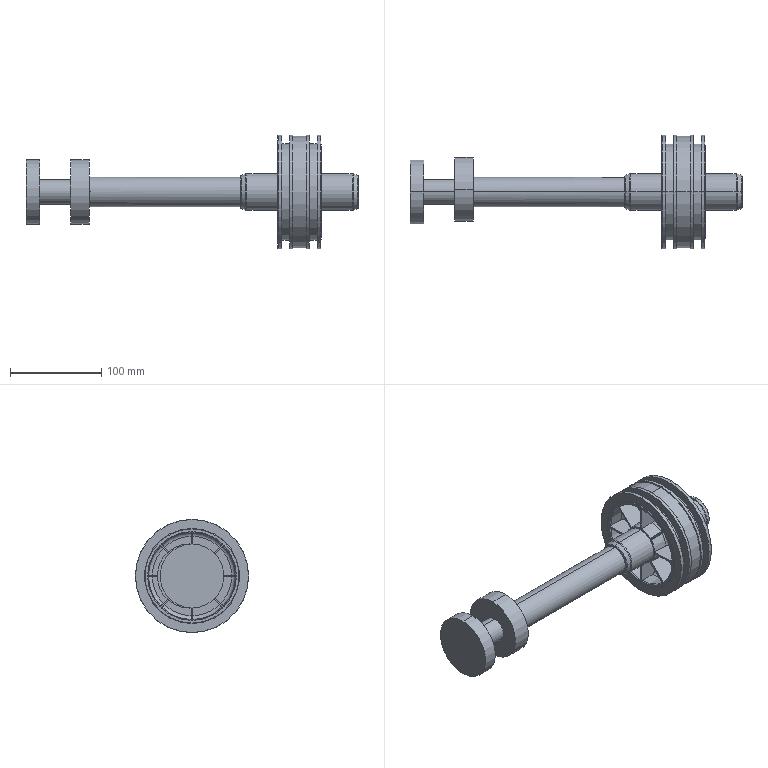Part | STEP file | 1 solid | 209 faces | box 363 x 124 x 124 mm | volume 637723 mm3 | plane 69 | torus 64 | cone 50 | cylinder 26 | commonest cylinder face diameters 124 x8 40 x4 70 x4 105 x4 27 x2 32 x2